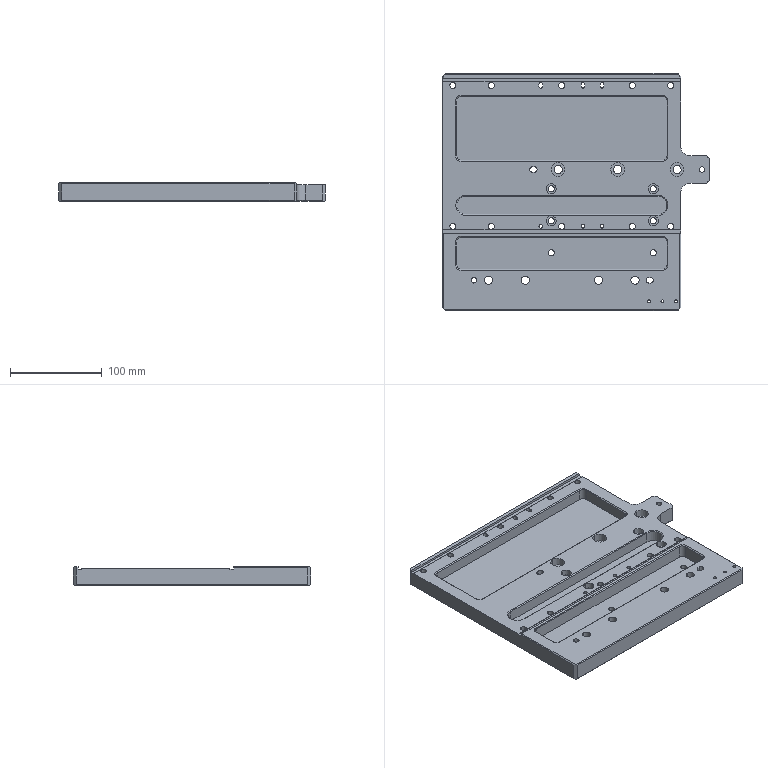Part | 1 solid | 233 faces | box 291 x 259 x 20 mm | volume 849567 mm3 | cylinder 129 | plane 92 | cone 12 | commonest cylinder face diameters 6.6 x32 11 x28 4 x15 9 x14 15 x14 6 x8